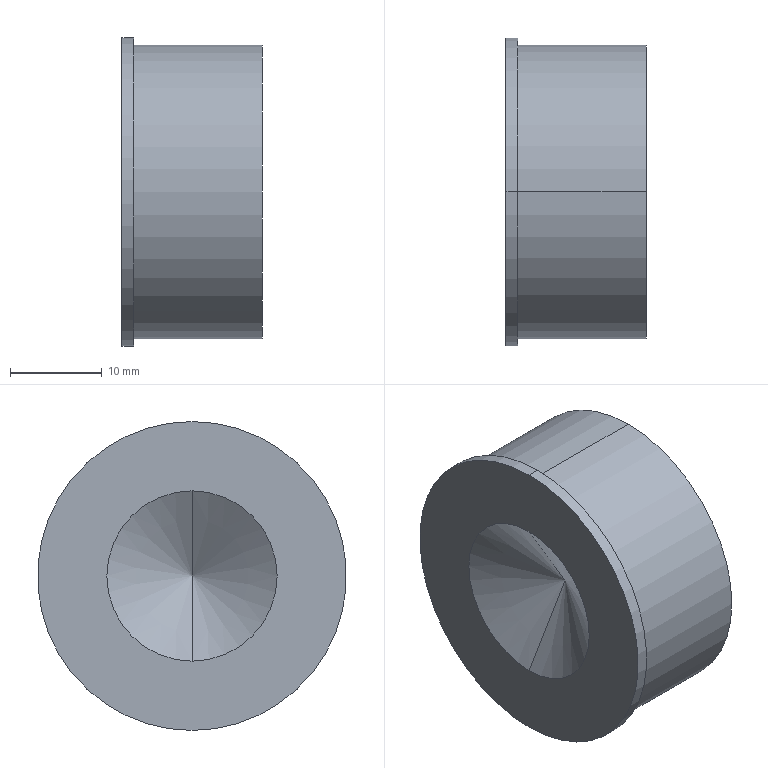Part | SolidWorks | features BaseBody 1 | 1 solid | 9 faces | box 15.3 x 33.7 x 33.7 mm | volume 11915 mm3 | cylinder 4 | plane 3 | cone 2 | commonest cylinder face diameters 32 x2 33.7 x2
STEP:
#1=CARTESIAN_POINT('',(223.5,-84.,173.621));
#2=VERTEX_POINT('',#1);
#3=CARTESIAN_POINT('',(223.5,-84.,205.621));
#4=VERTEX_POINT('',#3);
#5=CARTESIAN_POINT('',(223.5,-84.,189.621));
#6=DIRECTION('',(1.,0.,0.));
#7=DIRECTION('',(0.,0.,1.));
#8=AXIS2_PLACEMENT_3D('',#5,#6,#7);
#9=CIRCLE('',#8,16.);
#10=EDGE_CURVE('',#2,#4,#9,.T.);
#11=ORIENTED_EDGE('',*,*,#10,.F.);
#12=CARTESIAN_POINT('',(209.5,-84.,173.621));
#13=VERTEX_POINT('',#12);
#14=CARTESIAN_POINT('',(223.5,-84.,173.621));
#15=DIRECTION('',(-1.,0.,0.));
#16=VECTOR('',#15,1000.);
#17=LINE('',#14,#16);
#18=EDGE_CURVE('',#2,#13,#17,.T.);
#19=ORIENTED_EDGE('',*,*,#18,.T.);
#20=CARTESIAN_POINT('',(209.5,-84.,205.621));
#21=VERTEX_POINT('',#20);
#22=CARTESIAN_POINT('',(209.5,-84.,189.621));
#23=DIRECTION('',(1.,0.,0.));
#24=DIRECTION('',(0.,0.,1.));
#25=AXIS2_PLACEMENT_3D('',#22,#23,#24);
#26=CIRCLE('',#25,16.);
#27=EDGE_CURVE('',#13,#21,#26,.T.);
#28=ORIENTED_EDGE('',*,*,#27,.T.);
#29=CARTESIAN_POINT('',(223.5,-84.,205.621));
#30=DIRECTION('',(-1.,0.,0.));
#31=VECTOR('',#30,1000.);
#32=LINE('',#29,#31);
#33=EDGE_CURVE('',#4,#21,#32,.T.);
#34=ORIENTED_EDGE('',*,*,#33,.F.);
#35=EDGE_LOOP('',(#11,#19,#28,#34));
#36=FACE_OUTER_BOUND('',#35,.T.);
#37=CARTESIAN_POINT('',(223.5,-84.,189.621));
#38=DIRECTION('',(-1.,0.,0.));
#39=DIRECTION('',(0.,0.,1.));
#40=AXIS2_PLACEMENT_3D('',#37,#38,#39);
#41=CYLINDRICAL_SURFACE('',#40,16.);
#42=ADVANCED_FACE('',(#36),#41,.T.);
#43=CARTESIAN_POINT('',(209.5,-84.,172.771));
#44=VERTEX_POINT('',#43);
#45=CARTESIAN_POINT('',(209.5,-84.,206.471));
#46=VERTEX_POINT('',#45);
#47=CARTESIAN_POINT('',(209.5,-84.,189.621));
#48=DIRECTION('',(1.,0.,0.));
#49=DIRECTION('',(0.,0.,1.));
#50=AXIS2_PLACEMENT_3D('',#47,#48,#49);
#51=CIRCLE('',#50,16.85);
#52=EDGE_CURVE('',#44,#46,#51,.T.);
#53=ORIENTED_EDGE('',*,*,#52,.F.);
#54=CARTESIAN_POINT('',(208.2,-84.,172.771));
#55=VERTEX_POINT('',#54);
#56=CARTESIAN_POINT('',(209.5,-84.,172.771));
#57=DIRECTION('',(-1.,0.,0.));
#58=VECTOR('',#57,1000.);
#59=LINE('',#56,#58);
#60=EDGE_CURVE('',#44,#55,#59,.T.);
#61=ORIENTED_EDGE('',*,*,#60,.T.);
#62=CARTESIAN_POINT('',(208.2,-84.,206.471));
#63=VERTEX_POINT('',#62);
#64=CARTESIAN_POINT('',(208.2,-84.,189.621));
#65=DIRECTION('',(1.,0.,0.));
#66=DIRECTION('',(0.,0.,1.));
#67=AXIS2_PLACEMENT_3D('',#64,#65,#66);
#68=CIRCLE('',#67,16.85);
#69=EDGE_CURVE('',#55,#63,#68,.T.);
#70=ORIENTED_EDGE('',*,*,#69,.T.);
#71=CARTESIAN_POINT('',(209.5,-84.,206.471));
#72=DIRECTION('',(-1.,0.,0.));
#73=VECTOR('',#72,1000.);
#74=LINE('',#71,#73);
#75=EDGE_CURVE('',#46,#63,#74,.T.);
#76=ORIENTED_EDGE('',*,*,#75,.F.);
#77=EDGE_LOOP('',(#53,#61,#70,#76));
#78=FACE_OUTER_BOUND('',#77,.T.);
#79=CARTESIAN_POINT('',(209.5,-84.,189.621));
#80=DIRECTION('',(-1.,0.,0.));
#81=DIRECTION('',(0.,0.,1.));
#82=AXIS2_PLACEMENT_3D('',#79,#80,#81);
#83=CYLINDRICAL_SURFACE('',#82,16.85);
#84=ADVANCED_FACE('',(#78),#83,.T.);
#85=CARTESIAN_POINT('',(213.782,-84.,189.621));
#86=VERTEX_POINT('',#85);
#87=CARTESIAN_POINT('',(208.2,-84.,198.911));
#88=VERTEX_POINT('',#87);
#89=CARTESIAN_POINT('',(208.2,-84.,198.911));
#90=DIRECTION('',(-0.515,0.,0.8572));
#91=VECTOR('',#90,1000.);
#92=LINE('',#89,#91);
#93=EDGE_CURVE('',#86,#88,#92,.T.);
#94=ORIENTED_EDGE('',*,*,#93,.F.);
#95=CARTESIAN_POINT('',(208.2,-84.,180.331));
#96=VERTEX_POINT('',#95);
#97=CARTESIAN_POINT('',(208.2,-84.,180.331));
#98=DIRECTION('',(-0.515,0.,-0.8572));
#99=VECTOR('',#98,1000.);
#100=LINE('',#97,#99);
#101=EDGE_CURVE('',#86,#96,#100,.T.);
#102=ORIENTED_EDGE('',*,*,#101,.T.);
#103=CARTESIAN_POINT('',(208.2,-84.,189.621));
#104=DIRECTION('',(-1.,0.,0.));
#105=DIRECTION('',(0.,0.,1.));
#106=AXIS2_PLACEMENT_3D('',#103,#104,#105);
#107=CIRCLE('',#106,9.29);
#108=EDGE_CURVE('',#96,#88,#107,.T.);
#109=ORIENTED_EDGE('',*,*,#108,.T.);
#110=EDGE_LOOP('',(#94,#102,#109));
#111=FACE_OUTER_BOUND('',#110,.T.);
#112=CARTESIAN_POINT('',(208.2,-84.,189.621));
#113=DIRECTION('',(-1.,0.,0.));
#114=DIRECTION('',(0.,0.,1.));
#115=AXIS2_PLACEMENT_3D('',#112,#113,#114);
#116=CONICAL_SURFACE('',#115,9.29,1.03);
#117=ADVANCED_FACE('',(#111),#116,.F.);
#118=CARTESIAN_POINT('',(223.5,-84.,189.621));
#119=DIRECTION('',(1.,0.,0.));
#120=DIRECTION('',(0.,0.,1.));
#121=AXIS2_PLACEMENT_3D('',#118,#119,#120);
#122=CIRCLE('',#121,16.);
#123=EDGE_CURVE('',#4,#2,#122,.T.);
#124=ORIENTED_EDGE('',*,*,#123,.T.);
#125=ORIENTED_EDGE('',*,*,#10,.T.);
#126=EDGE_LOOP('',(#124,#125));
#127=FACE_OUTER_BOUND('',#126,.T.);
#128=CARTESIAN_POINT('',(223.5,-84.,189.621));
#129=DIRECTION('',(1.,0.,0.));
#130=DIRECTION('',(0.,0.,-1.));
#131=AXIS2_PLACEMENT_3D('',#128,#129,#130);
#132=PLANE('',#131);
#133=ADVANCED_FACE('',(#127),#132,.T.);
#134=ORIENTED_EDGE('',*,*,#18,.F.);
#135=ORIENTED_EDGE('',*,*,#123,.F.);
#136=ORIENTED_EDGE('',*,*,#33,.T.);
#137=CARTESIAN_POINT('',(209.5,-84.,189.621));
#138=DIRECTION('',(1.,0.,0.));
#139=DIRECTION('',(0.,0.,1.));
#140=AXIS2_PLACEMENT_3D('',#137,#138,#139);
#141=CIRCLE('',#140,16.);
#142=EDGE_CURVE('',#21,#13,#141,.T.);
#143=ORIENTED_EDGE('',*,*,#142,.T.);
#144=EDGE_LOOP('',(#134,#135,#136,#143));
#145=FACE_OUTER_BOUND('',#144,.T.);
#146=CARTESIAN_POINT('',(223.5,-84.,189.621));
#147=DIRECTION('',(-1.,0.,0.));
#148=DIRECTION('',(0.,0.,1.));
#149=AXIS2_PLACEMENT_3D('',#146,#147,#148);
#150=CYLINDRICAL_SURFACE('',#149,16.);
#151=ADVANCED_FACE('',(#145),#150,.T.);
#152=ORIENTED_EDGE('',*,*,#142,.F.);
#153=ORIENTED_EDGE('',*,*,#27,.F.);
#154=EDGE_LOOP('',(#152,#153));
#155=FACE_BOUND('',#154,.T.);
#156=CARTESIAN_POINT('',(209.5,-84.,189.621));
#157=DIRECTION('',(1.,0.,0.));
#158=DIRECTION('',(0.,0.,1.));
#159=AXIS2_PLACEMENT_3D('',#156,#157,#158);
#160=CIRCLE('',#159,16.85);
#161=EDGE_CURVE('',#46,#44,#160,.T.);
#162=ORIENTED_EDGE('',*,*,#161,.T.);
#163=ORIENTED_EDGE('',*,*,#52,.T.);
#164=EDGE_LOOP('',(#162,#163));
#165=FACE_OUTER_BOUND('',#164,.T.);
#166=CARTESIAN_POINT('',(209.5,-84.,189.621));
#167=DIRECTION('',(1.,0.,0.));
#168=DIRECTION('',(0.,0.,-1.));
#169=AXIS2_PLACEMENT_3D('',#166,#167,#168);
#170=PLANE('',#169);
#171=ADVANCED_FACE('',(#155,#165),#170,.T.);
#172=ORIENTED_EDGE('',*,*,#60,.F.);
#173=ORIENTED_EDGE('',*,*,#161,.F.);
#174=ORIENTED_EDGE('',*,*,#75,.T.);
#175=CARTESIAN_POINT('',(208.2,-84.,189.621));
#176=DIRECTION('',(1.,0.,0.));
#177=DIRECTION('',(0.,0.,1.));
#178=AXIS2_PLACEMENT_3D('',#175,#176,#177);
#179=CIRCLE('',#178,16.85);
#180=EDGE_CURVE('',#63,#55,#179,.T.);
#181=ORIENTED_EDGE('',*,*,#180,.T.);
#182=EDGE_LOOP('',(#172,#173,#174,#181));
#183=FACE_OUTER_BOUND('',#182,.T.);
#184=CARTESIAN_POINT('',(209.5,-84.,189.621));
#185=DIRECTION('',(-1.,0.,0.));
#186=DIRECTION('',(0.,0.,1.));
#187=AXIS2_PLACEMENT_3D('',#184,#185,#186);
#188=CYLINDRICAL_SURFACE('',#187,16.85);
#189=ADVANCED_FACE('',(#183),#188,.T.);
#190=CARTESIAN_POINT('',(208.2,-84.,189.621));
#191=DIRECTION('',(-1.,0.,0.));
#192=DIRECTION('',(0.,0.,1.));
#193=AXIS2_PLACEMENT_3D('',#190,#191,#192);
#194=CIRCLE('',#193,9.29);
#195=EDGE_CURVE('',#88,#96,#194,.T.);
#196=ORIENTED_EDGE('',*,*,#195,.F.);
#197=ORIENTED_EDGE('',*,*,#108,.F.);
#198=EDGE_LOOP('',(#196,#197));
#199=FACE_BOUND('',#198,.T.);
#200=ORIENTED_EDGE('',*,*,#180,.F.);
#201=ORIENTED_EDGE('',*,*,#69,.F.);
#202=EDGE_LOOP('',(#200,#201));
#203=FACE_OUTER_BOUND('',#202,.T.);
#204=CARTESIAN_POINT('',(208.2,-84.,189.621));
#205=DIRECTION('',(1.,0.,0.));
#206=DIRECTION('',(0.,0.,-1.));
#207=AXIS2_PLACEMENT_3D('',#204,#205,#206);
#208=PLANE('',#207);
#209=ADVANCED_FACE('',(#199,#203),#208,.F.);
#210=ORIENTED_EDGE('',*,*,#101,.F.);
#211=ORIENTED_EDGE('',*,*,#93,.T.);
#212=ORIENTED_EDGE('',*,*,#195,.T.);
#213=EDGE_LOOP('',(#210,#211,#212));
#214=FACE_OUTER_BOUND('',#213,.T.);
#215=CARTESIAN_POINT('',(208.2,-84.,189.621));
#216=DIRECTION('',(-1.,0.,0.));
#217=DIRECTION('',(0.,0.,1.));
#218=AXIS2_PLACEMENT_3D('',#215,#216,#217);
#219=CONICAL_SURFACE('',#218,9.29,1.03);
#220=ADVANCED_FACE('',(#214),#219,.F.);
#221=CLOSED_SHELL('',(#42,#84,#117,#133,#151,#171,#189,#209,#220));
#222=MANIFOLD_SOLID_BREP('',#221);
#223=CARTESIAN_POINT('',(0.,0.,0.));
#224=DIRECTION('',(0.,0.,1.));
#225=DIRECTION('',(1.,0.,0.));
#226=AXIS2_PLACEMENT_3D('',#223,#224,#225);
#227=(LENGTH_UNIT()NAMED_UNIT(*)SI_UNIT(.MILLI.,.METRE.));
#228=UNCERTAINTY_MEASURE_WITH_UNIT(LENGTH_MEASURE(0.00001),#227,'','');
#229=(NAMED_UNIT(*)PLANE_ANGLE_UNIT()SI_UNIT($,.RADIAN.));
#230=(NAMED_UNIT(*)SI_UNIT($,.STERADIAN.)SOLID_ANGLE_UNIT());
#231=(GEOMETRIC_REPRESENTATION_CONTEXT(3)GLOBAL_UNCERTAINTY_ASSIGNED_CONTEXT((#228))GLOBAL_UNIT_ASSIGNED_CONTEXT((#227,#229,#230))REPRESENTATION_CONTEXT('',''));
#232=ADVANCED_BREP_SHAPE_REPRESENTATION('',(#222,#226),#231);